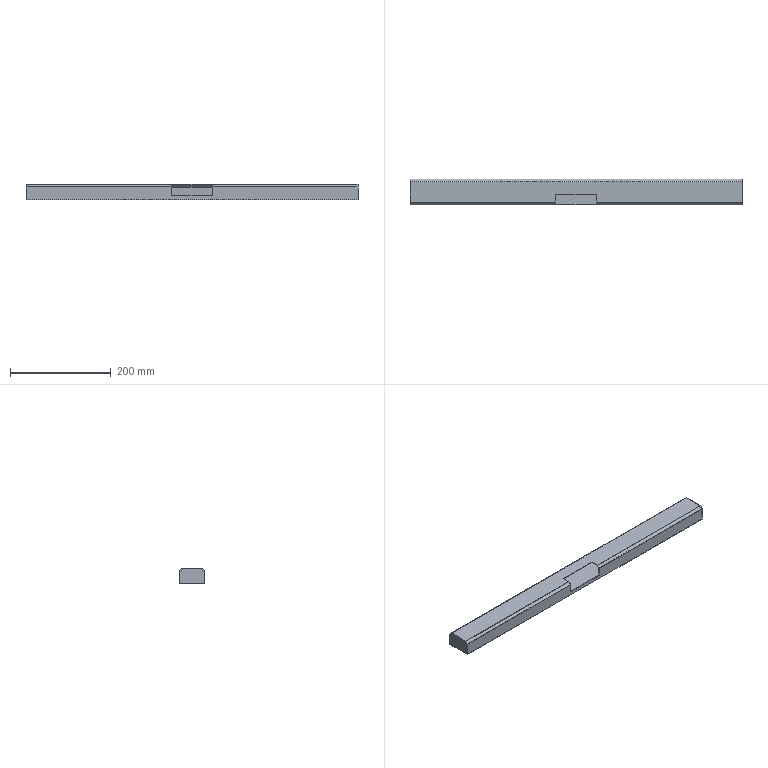Part | STEP file | Guide wheel mechanism revised.sldasm-Part-190 | 1 solid | 22 faces | box 660 x 50 x 30 mm | volume 98910 mm3 | plane 22
STEP:
#1=CARTESIAN_POINT('',(40.,-20.5,108.));
#2=VERTEX_POINT('',#1);
#3=CARTESIAN_POINT('',(40.,-20.5,124.586));
#4=VERTEX_POINT('',#3);
#5=CARTESIAN_POINT('',(40.,-20.5,133.));
#6=DIRECTION('',(0.,0.,1.));
#7=VECTOR('',#6,1000.);
#8=LINE('',#5,#7);
#9=EDGE_CURVE('',#2,#4,#8,.T.);
#10=ORIENTED_EDGE('',*,*,#9,.F.);
#11=CARTESIAN_POINT('',(40.,-21.5,108.));
#12=VERTEX_POINT('',#11);
#13=CARTESIAN_POINT('',(40.,-1.5,108.));
#14=DIRECTION('',(0.,-1.,0.));
#15=VECTOR('',#14,1000.);
#16=LINE('',#13,#15);
#17=EDGE_CURVE('',#2,#12,#16,.T.);
#18=ORIENTED_EDGE('',*,*,#17,.T.);
#19=CARTESIAN_POINT('',(40.,-21.5,125.));
#20=VERTEX_POINT('',#19);
#21=CARTESIAN_POINT('',(40.,-21.5,133.));
#22=DIRECTION('',(0.,0.,1.));
#23=VECTOR('',#22,1000.);
#24=LINE('',#21,#23);
#25=EDGE_CURVE('',#12,#20,#24,.T.);
#26=ORIENTED_EDGE('',*,*,#25,.T.);
#27=CARTESIAN_POINT('',(40.,-16.5,130.));
#28=VERTEX_POINT('',#27);
#29=CARTESIAN_POINT('',(40.,-21.5,125.));
#30=DIRECTION('',(0.,-0.7071,-0.7071));
#31=VECTOR('',#30,1000.);
#32=LINE('',#29,#31);
#33=EDGE_CURVE('',#28,#20,#32,.T.);
#34=ORIENTED_EDGE('',*,*,#33,.F.);
#35=CARTESIAN_POINT('',(40.,-1.5,130.));
#36=VERTEX_POINT('',#35);
#37=CARTESIAN_POINT('',(40.,-16.5,130.));
#38=DIRECTION('',(0.,-1.,0.));
#39=VECTOR('',#38,1000.);
#40=LINE('',#37,#39);
#41=EDGE_CURVE('',#36,#28,#40,.T.);
#42=ORIENTED_EDGE('',*,*,#41,.F.);
#43=CARTESIAN_POINT('',(40.,-1.5,129.));
#44=VERTEX_POINT('',#43);
#45=CARTESIAN_POINT('',(40.,-1.5,133.));
#46=DIRECTION('',(0.,0.,1.));
#47=VECTOR('',#46,1000.);
#48=LINE('',#45,#47);
#49=EDGE_CURVE('',#44,#36,#48,.T.);
#50=ORIENTED_EDGE('',*,*,#49,.F.);
#51=CARTESIAN_POINT('',(40.,-16.086,129.));
#52=VERTEX_POINT('',#51);
#53=CARTESIAN_POINT('',(40.,-16.5,129.));
#54=DIRECTION('',(0.,-1.,0.));
#55=VECTOR('',#54,1000.);
#56=LINE('',#53,#55);
#57=EDGE_CURVE('',#44,#52,#56,.T.);
#58=ORIENTED_EDGE('',*,*,#57,.T.);
#59=CARTESIAN_POINT('',(40.,-20.793,124.293));
#60=DIRECTION('',(0.,-0.7071,-0.7071));
#61=VECTOR('',#60,1000.);
#62=LINE('',#59,#61);
#63=EDGE_CURVE('',#52,#4,#62,.T.);
#64=ORIENTED_EDGE('',*,*,#63,.T.);
#65=EDGE_LOOP('',(#10,#18,#26,#34,#42,#50,#58,#64));
#66=FACE_OUTER_BOUND('',#65,.T.);
#67=CARTESIAN_POINT('',(40.,-1.5,133.));
#68=DIRECTION('',(1.,0.,0.));
#69=DIRECTION('',(0.,0.,-1.));
#70=AXIS2_PLACEMENT_3D('',#67,#68,#69);
#71=PLANE('',#70);
#72=ADVANCED_FACE('',(#66),#71,.F.);
#73=CARTESIAN_POINT('',(-40.,-20.5,108.));
#74=VERTEX_POINT('',#73);
#75=CARTESIAN_POINT('',(-40.,-20.5,108.));
#76=DIRECTION('',(1.,0.,0.));
#77=VECTOR('',#76,1000.);
#78=LINE('',#75,#77);
#79=EDGE_CURVE('',#74,#2,#78,.T.);
#80=ORIENTED_EDGE('',*,*,#79,.F.);
#81=CARTESIAN_POINT('',(-40.,-21.5,108.));
#82=VERTEX_POINT('',#81);
#83=CARTESIAN_POINT('',(-40.,-1.5,108.));
#84=DIRECTION('',(0.,-1.,0.));
#85=VECTOR('',#84,1000.);
#86=LINE('',#83,#85);
#87=EDGE_CURVE('',#74,#82,#86,.T.);
#88=ORIENTED_EDGE('',*,*,#87,.T.);
#89=CARTESIAN_POINT('',(-40.,-21.5,108.));
#90=DIRECTION('',(1.,0.,0.));
#91=VECTOR('',#90,1000.);
#92=LINE('',#89,#91);
#93=EDGE_CURVE('',#82,#12,#92,.T.);
#94=ORIENTED_EDGE('',*,*,#93,.T.);
#95=ORIENTED_EDGE('',*,*,#17,.F.);
#96=EDGE_LOOP('',(#80,#88,#94,#95));
#97=FACE_OUTER_BOUND('',#96,.T.);
#98=CARTESIAN_POINT('',(-40.,-1.5,108.));
#99=DIRECTION('',(0.,0.,-1.));
#100=DIRECTION('',(0.,1.,0.));
#101=AXIS2_PLACEMENT_3D('',#98,#99,#100);
#102=PLANE('',#101);
#103=ADVANCED_FACE('',(#97),#102,.F.);
#104=CARTESIAN_POINT('',(-40.,-21.5,125.));
#105=VERTEX_POINT('',#104);
#106=CARTESIAN_POINT('',(-330.,-21.5,125.));
#107=VERTEX_POINT('',#106);
#108=CARTESIAN_POINT('',(330.,-21.5,125.));
#109=DIRECTION('',(-1.,0.,0.));
#110=VECTOR('',#109,1000.);
#111=LINE('',#108,#110);
#112=EDGE_CURVE('',#105,#107,#111,.T.);
#113=ORIENTED_EDGE('',*,*,#112,.F.);
#114=CARTESIAN_POINT('',(-40.,-16.5,130.));
#115=VERTEX_POINT('',#114);
#116=CARTESIAN_POINT('',(-40.,-21.5,125.));
#117=DIRECTION('',(0.,0.7071,0.7071));
#118=VECTOR('',#117,1000.);
#119=LINE('',#116,#118);
#120=EDGE_CURVE('',#105,#115,#119,.T.);
#121=ORIENTED_EDGE('',*,*,#120,.T.);
#122=CARTESIAN_POINT('',(-330.,-16.5,130.));
#123=VERTEX_POINT('',#122);
#124=CARTESIAN_POINT('',(330.,-16.5,130.));
#125=DIRECTION('',(-1.,0.,0.));
#126=VECTOR('',#125,1000.);
#127=LINE('',#124,#126);
#128=EDGE_CURVE('',#115,#123,#127,.T.);
#129=ORIENTED_EDGE('',*,*,#128,.T.);
#130=CARTESIAN_POINT('',(-330.,-21.5,125.));
#131=DIRECTION('',(0.,-0.7071,-0.7071));
#132=VECTOR('',#131,1000.);
#133=LINE('',#130,#132);
#134=EDGE_CURVE('',#123,#107,#133,.T.);
#135=ORIENTED_EDGE('',*,*,#134,.T.);
#136=EDGE_LOOP('',(#113,#121,#129,#135));
#137=FACE_OUTER_BOUND('',#136,.T.);
#138=CARTESIAN_POINT('',(330.,-21.5,125.));
#139=DIRECTION('',(0.,0.7071,-0.7071));
#140=DIRECTION('',(0.,0.7071,0.7071));
#141=AXIS2_PLACEMENT_3D('',#138,#139,#140);
#142=PLANE('',#141);
#143=ADVANCED_FACE('',(#137),#142,.F.);
#144=CARTESIAN_POINT('',(-330.,28.5,100.));
#145=VERTEX_POINT('',#144);
#146=CARTESIAN_POINT('',(-330.,28.5,125.));
#147=VERTEX_POINT('',#146);
#148=CARTESIAN_POINT('',(-330.,28.5,125.));
#149=DIRECTION('',(0.,0.,1.));
#150=VECTOR('',#149,1000.);
#151=LINE('',#148,#150);
#152=EDGE_CURVE('',#145,#147,#151,.T.);
#153=ORIENTED_EDGE('',*,*,#152,.T.);
#154=CARTESIAN_POINT('',(330.,28.5,125.));
#155=VERTEX_POINT('',#154);
#156=CARTESIAN_POINT('',(330.,28.5,125.));
#157=DIRECTION('',(-1.,0.,0.));
#158=VECTOR('',#157,1000.);
#159=LINE('',#156,#158);
#160=EDGE_CURVE('',#155,#147,#159,.T.);
#161=ORIENTED_EDGE('',*,*,#160,.F.);
#162=CARTESIAN_POINT('',(330.,28.5,100.));
#163=VERTEX_POINT('',#162);
#164=CARTESIAN_POINT('',(330.,28.5,125.));
#165=DIRECTION('',(0.,0.,1.));
#166=VECTOR('',#165,1000.);
#167=LINE('',#164,#166);
#168=EDGE_CURVE('',#163,#155,#167,.T.);
#169=ORIENTED_EDGE('',*,*,#168,.F.);
#170=CARTESIAN_POINT('',(330.,28.5,100.));
#171=DIRECTION('',(-1.,0.,0.));
#172=VECTOR('',#171,1000.);
#173=LINE('',#170,#172);
#174=EDGE_CURVE('',#163,#145,#173,.T.);
#175=ORIENTED_EDGE('',*,*,#174,.T.);
#176=EDGE_LOOP('',(#153,#161,#169,#175));
#177=FACE_OUTER_BOUND('',#176,.T.);
#178=CARTESIAN_POINT('',(330.,28.5,125.));
#179=DIRECTION('',(0.,-1.,0.));
#180=DIRECTION('',(0.,0.,-1.));
#181=AXIS2_PLACEMENT_3D('',#178,#179,#180);
#182=PLANE('',#181);
#183=ADVANCED_FACE('',(#177),#182,.F.);
#184=CARTESIAN_POINT('',(-330.,23.5,130.));
#185=VERTEX_POINT('',#184);
#186=CARTESIAN_POINT('',(-330.,23.5,130.));
#187=DIRECTION('',(0.,-0.7071,0.7071));
#188=VECTOR('',#187,1000.);
#189=LINE('',#186,#188);
#190=EDGE_CURVE('',#147,#185,#189,.T.);
#191=ORIENTED_EDGE('',*,*,#190,.T.);
#192=CARTESIAN_POINT('',(330.,23.5,130.));
#193=VERTEX_POINT('',#192);
#194=CARTESIAN_POINT('',(330.,23.5,130.));
#195=DIRECTION('',(-1.,0.,0.));
#196=VECTOR('',#195,1000.);
#197=LINE('',#194,#196);
#198=EDGE_CURVE('',#193,#185,#197,.T.);
#199=ORIENTED_EDGE('',*,*,#198,.F.);
#200=CARTESIAN_POINT('',(330.,23.5,130.));
#201=DIRECTION('',(0.,-0.7071,0.7071));
#202=VECTOR('',#201,1000.);
#203=LINE('',#200,#202);
#204=EDGE_CURVE('',#155,#193,#203,.T.);
#205=ORIENTED_EDGE('',*,*,#204,.F.);
#206=ORIENTED_EDGE('',*,*,#160,.T.);
#207=EDGE_LOOP('',(#191,#199,#205,#206));
#208=FACE_OUTER_BOUND('',#207,.T.);
#209=CARTESIAN_POINT('',(330.,23.5,130.));
#210=DIRECTION('',(0.,-0.7071,-0.7071));
#211=DIRECTION('',(0.,0.7071,-0.7071));
#212=AXIS2_PLACEMENT_3D('',#209,#210,#211);
#213=PLANE('',#212);
#214=ADVANCED_FACE('',(#208),#213,.F.);
#215=ORIENTED_EDGE('',*,*,#128,.F.);
#216=CARTESIAN_POINT('',(-40.,-1.5,130.));
#217=VERTEX_POINT('',#216);
#218=CARTESIAN_POINT('',(-40.,-16.5,130.));
#219=DIRECTION('',(0.,1.,0.));
#220=VECTOR('',#219,1000.);
#221=LINE('',#218,#220);
#222=EDGE_CURVE('',#115,#217,#221,.T.);
#223=ORIENTED_EDGE('',*,*,#222,.T.);
#224=CARTESIAN_POINT('',(330.,-1.5,130.));
#225=DIRECTION('',(-1.,0.,0.));
#226=VECTOR('',#225,1000.);
#227=LINE('',#224,#226);
#228=EDGE_CURVE('',#36,#217,#227,.T.);
#229=ORIENTED_EDGE('',*,*,#228,.F.);
#230=ORIENTED_EDGE('',*,*,#41,.T.);
#231=CARTESIAN_POINT('',(330.,-16.5,130.));
#232=VERTEX_POINT('',#231);
#233=CARTESIAN_POINT('',(330.,-16.5,130.));
#234=DIRECTION('',(-1.,0.,0.));
#235=VECTOR('',#234,1000.);
#236=LINE('',#233,#235);
#237=EDGE_CURVE('',#232,#28,#236,.T.);
#238=ORIENTED_EDGE('',*,*,#237,.F.);
#239=CARTESIAN_POINT('',(330.,-16.5,130.));
#240=DIRECTION('',(0.,-1.,0.));
#241=VECTOR('',#240,1000.);
#242=LINE('',#239,#241);
#243=EDGE_CURVE('',#193,#232,#242,.T.);
#244=ORIENTED_EDGE('',*,*,#243,.F.);
#245=ORIENTED_EDGE('',*,*,#198,.T.);
#246=CARTESIAN_POINT('',(-330.,-16.5,130.));
#247=DIRECTION('',(0.,-1.,0.));
#248=VECTOR('',#247,1000.);
#249=LINE('',#246,#248);
#250=EDGE_CURVE('',#185,#123,#249,.T.);
#251=ORIENTED_EDGE('',*,*,#250,.T.);
#252=EDGE_LOOP('',(#215,#223,#229,#230,#238,#244,#245,#251));
#253=FACE_OUTER_BOUND('',#252,.T.);
#254=CARTESIAN_POINT('',(330.,-16.5,130.));
#255=DIRECTION('',(0.,0.,-1.));
#256=DIRECTION('',(0.,1.,0.));
#257=AXIS2_PLACEMENT_3D('',#254,#255,#256);
#258=PLANE('',#257);
#259=ADVANCED_FACE('',(#253),#258,.F.);
#260=ORIENTED_EDGE('',*,*,#237,.T.);
#261=ORIENTED_EDGE('',*,*,#33,.T.);
#262=CARTESIAN_POINT('',(330.,-21.5,125.));
#263=VERTEX_POINT('',#262);
#264=CARTESIAN_POINT('',(330.,-21.5,125.));
#265=DIRECTION('',(-1.,0.,0.));
#266=VECTOR('',#265,1000.);
#267=LINE('',#264,#266);
#268=EDGE_CURVE('',#263,#20,#267,.T.);
#269=ORIENTED_EDGE('',*,*,#268,.F.);
#270=CARTESIAN_POINT('',(330.,-21.5,125.));
#271=DIRECTION('',(0.,-0.7071,-0.7071));
#272=VECTOR('',#271,1000.);
#273=LINE('',#270,#272);
#274=EDGE_CURVE('',#232,#263,#273,.T.);
#275=ORIENTED_EDGE('',*,*,#274,.F.);
#276=EDGE_LOOP('',(#260,#261,#269,#275));
#277=FACE_OUTER_BOUND('',#276,.T.);
#278=CARTESIAN_POINT('',(330.,-21.5,125.));
#279=DIRECTION('',(0.,0.7071,-0.7071));
#280=DIRECTION('',(0.,0.7071,0.7071));
#281=AXIS2_PLACEMENT_3D('',#278,#279,#280);
#282=PLANE('',#281);
#283=ADVANCED_FACE('',(#277),#282,.F.);
#284=ORIENTED_EDGE('',*,*,#93,.F.);
#285=CARTESIAN_POINT('',(-40.,-21.5,100.));
#286=DIRECTION('',(0.,0.,1.));
#287=VECTOR('',#286,1000.);
#288=LINE('',#285,#287);
#289=EDGE_CURVE('',#82,#105,#288,.T.);
#290=ORIENTED_EDGE('',*,*,#289,.T.);
#291=ORIENTED_EDGE('',*,*,#112,.T.);
#292=CARTESIAN_POINT('',(-330.,-21.5,100.));
#293=VERTEX_POINT('',#292);
#294=CARTESIAN_POINT('',(-330.,-21.5,100.));
#295=DIRECTION('',(0.,0.,-1.));
#296=VECTOR('',#295,1000.);
#297=LINE('',#294,#296);
#298=EDGE_CURVE('',#107,#293,#297,.T.);
#299=ORIENTED_EDGE('',*,*,#298,.T.);
#300=CARTESIAN_POINT('',(330.,-21.5,100.));
#301=VERTEX_POINT('',#300);
#302=CARTESIAN_POINT('',(330.,-21.5,100.));
#303=DIRECTION('',(-1.,0.,0.));
#304=VECTOR('',#303,1000.);
#305=LINE('',#302,#304);
#306=EDGE_CURVE('',#301,#293,#305,.T.);
#307=ORIENTED_EDGE('',*,*,#306,.F.);
#308=CARTESIAN_POINT('',(330.,-21.5,100.));
#309=DIRECTION('',(0.,0.,-1.));
#310=VECTOR('',#309,1000.);
#311=LINE('',#308,#310);
#312=EDGE_CURVE('',#263,#301,#311,.T.);
#313=ORIENTED_EDGE('',*,*,#312,.F.);
#314=ORIENTED_EDGE('',*,*,#268,.T.);
#315=ORIENTED_EDGE('',*,*,#25,.F.);
#316=EDGE_LOOP('',(#284,#290,#291,#299,#307,#313,#314,#315));
#317=FACE_OUTER_BOUND('',#316,.T.);
#318=CARTESIAN_POINT('',(330.,-21.5,100.));
#319=DIRECTION('',(0.,1.,0.));
#320=DIRECTION('',(0.,0.,1.));
#321=AXIS2_PLACEMENT_3D('',#318,#319,#320);
#322=PLANE('',#321);
#323=ADVANCED_FACE('',(#317),#322,.F.);
#324=CARTESIAN_POINT('',(-330.,28.5,100.));
#325=DIRECTION('',(0.,1.,0.));
#326=VECTOR('',#325,1000.);
#327=LINE('',#324,#326);
#328=EDGE_CURVE('',#293,#145,#327,.T.);
#329=ORIENTED_EDGE('',*,*,#328,.T.);
#330=ORIENTED_EDGE('',*,*,#174,.F.);
#331=CARTESIAN_POINT('',(330.,28.5,100.));
#332=DIRECTION('',(0.,1.,0.));
#333=VECTOR('',#332,1000.);
#334=LINE('',#331,#333);
#335=EDGE_CURVE('',#301,#163,#334,.T.);
#336=ORIENTED_EDGE('',*,*,#335,.F.);
#337=ORIENTED_EDGE('',*,*,#306,.T.);
#338=EDGE_LOOP('',(#329,#330,#336,#337));
#339=FACE_OUTER_BOUND('',#338,.T.);
#340=CARTESIAN_POINT('',(330.,28.5,100.));
#341=DIRECTION('',(0.,0.,1.));
#342=DIRECTION('',(0.,-1.,0.));
#343=AXIS2_PLACEMENT_3D('',#340,#341,#342);
#344=PLANE('',#343);
#345=ADVANCED_FACE('',(#339),#344,.F.);
#346=ORIENTED_EDGE('',*,*,#168,.T.);
#347=ORIENTED_EDGE('',*,*,#204,.T.);
#348=ORIENTED_EDGE('',*,*,#243,.T.);
#349=ORIENTED_EDGE('',*,*,#274,.T.);
#350=ORIENTED_EDGE('',*,*,#312,.T.);
#351=ORIENTED_EDGE('',*,*,#335,.T.);
#352=EDGE_LOOP('',(#346,#347,#348,#349,#350,#351));
#353=FACE_OUTER_BOUND('',#352,.T.);
#354=CARTESIAN_POINT('',(330.,28.5,100.));
#355=DIRECTION('',(-1.,0.,0.));
#356=DIRECTION('',(0.,0.,1.));
#357=AXIS2_PLACEMENT_3D('',#354,#355,#356);
#358=PLANE('',#357);
#359=ADVANCED_FACE('',(#353),#358,.F.);
#360=ORIENTED_EDGE('',*,*,#152,.F.);
#361=ORIENTED_EDGE('',*,*,#328,.F.);
#362=ORIENTED_EDGE('',*,*,#298,.F.);
#363=ORIENTED_EDGE('',*,*,#134,.F.);
#364=ORIENTED_EDGE('',*,*,#250,.F.);
#365=ORIENTED_EDGE('',*,*,#190,.F.);
#366=EDGE_LOOP('',(#360,#361,#362,#363,#364,#365));
#367=FACE_OUTER_BOUND('',#366,.T.);
#368=CARTESIAN_POINT('',(-330.,28.5,100.));
#369=DIRECTION('',(-1.,0.,0.));
#370=DIRECTION('',(0.,0.,1.));
#371=AXIS2_PLACEMENT_3D('',#368,#369,#370);
#372=PLANE('',#371);
#373=ADVANCED_FACE('',(#367),#372,.T.);
#374=CARTESIAN_POINT('',(-40.,-1.5,129.));
#375=VERTEX_POINT('',#374);
#376=CARTESIAN_POINT('',(330.,-1.5,129.));
#377=DIRECTION('',(-1.,0.,0.));
#378=VECTOR('',#377,1000.);
#379=LINE('',#376,#378);
#380=EDGE_CURVE('',#44,#375,#379,.T.);
#381=ORIENTED_EDGE('',*,*,#380,.F.);
#382=ORIENTED_EDGE('',*,*,#49,.T.);
#383=ORIENTED_EDGE('',*,*,#228,.T.);
#384=CARTESIAN_POINT('',(-40.,-1.5,133.));
#385=DIRECTION('',(0.,0.,-1.));
#386=VECTOR('',#385,1000.);
#387=LINE('',#384,#386);
#388=EDGE_CURVE('',#217,#375,#387,.T.);
#389=ORIENTED_EDGE('',*,*,#388,.T.);
#390=EDGE_LOOP('',(#381,#382,#383,#389));
#391=FACE_OUTER_BOUND('',#390,.T.);
#392=CARTESIAN_POINT('',(-40.,-1.5,108.));
#393=DIRECTION('',(0.,-1.,0.));
#394=DIRECTION('',(0.,0.,-1.));
#395=AXIS2_PLACEMENT_3D('',#392,#393,#394);
#396=PLANE('',#395);
#397=ADVANCED_FACE('',(#391),#396,.T.);
#398=ORIENTED_EDGE('',*,*,#87,.F.);
#399=CARTESIAN_POINT('',(-40.,-20.5,124.586));
#400=VERTEX_POINT('',#399);
#401=CARTESIAN_POINT('',(-40.,-20.5,100.));
#402=DIRECTION('',(0.,0.,1.));
#403=VECTOR('',#402,1000.);
#404=LINE('',#401,#403);
#405=EDGE_CURVE('',#74,#400,#404,.T.);
#406=ORIENTED_EDGE('',*,*,#405,.T.);
#407=CARTESIAN_POINT('',(-40.,-16.086,129.));
#408=VERTEX_POINT('',#407);
#409=CARTESIAN_POINT('',(-40.,-20.793,124.293));
#410=DIRECTION('',(0.,0.7071,0.7071));
#411=VECTOR('',#410,1000.);
#412=LINE('',#409,#411);
#413=EDGE_CURVE('',#400,#408,#412,.T.);
#414=ORIENTED_EDGE('',*,*,#413,.T.);
#415=CARTESIAN_POINT('',(-40.,-16.5,129.));
#416=DIRECTION('',(0.,1.,0.));
#417=VECTOR('',#416,1000.);
#418=LINE('',#415,#417);
#419=EDGE_CURVE('',#408,#375,#418,.T.);
#420=ORIENTED_EDGE('',*,*,#419,.T.);
#421=ORIENTED_EDGE('',*,*,#388,.F.);
#422=ORIENTED_EDGE('',*,*,#222,.F.);
#423=ORIENTED_EDGE('',*,*,#120,.F.);
#424=ORIENTED_EDGE('',*,*,#289,.F.);
#425=EDGE_LOOP('',(#398,#406,#414,#420,#421,#422,#423,#424));
#426=FACE_OUTER_BOUND('',#425,.T.);
#427=CARTESIAN_POINT('',(-40.,-1.5,133.));
#428=DIRECTION('',(-1.,0.,0.));
#429=DIRECTION('',(0.,0.,1.));
#430=AXIS2_PLACEMENT_3D('',#427,#428,#429);
#431=PLANE('',#430);
#432=ADVANCED_FACE('',(#426),#431,.F.);
#433=CARTESIAN_POINT('',(-329.,-20.5,124.586));
#434=VERTEX_POINT('',#433);
#435=CARTESIAN_POINT('',(330.,-20.5,124.586));
#436=DIRECTION('',(-1.,0.,0.));
#437=VECTOR('',#436,1000.);
#438=LINE('',#435,#437);
#439=EDGE_CURVE('',#400,#434,#438,.T.);
#440=ORIENTED_EDGE('',*,*,#439,.T.);
#441=CARTESIAN_POINT('',(-329.,-16.086,129.));
#442=VERTEX_POINT('',#441);
#443=CARTESIAN_POINT('',(-329.,-8.293,136.793));
#444=DIRECTION('',(0.,-0.7071,-0.7071));
#445=VECTOR('',#444,1000.);
#446=LINE('',#443,#445);
#447=EDGE_CURVE('',#442,#434,#446,.T.);
#448=ORIENTED_EDGE('',*,*,#447,.F.);
#449=CARTESIAN_POINT('',(330.,-16.086,129.));
#450=DIRECTION('',(-1.,0.,0.));
#451=VECTOR('',#450,1000.);
#452=LINE('',#449,#451);
#453=EDGE_CURVE('',#408,#442,#452,.T.);
#454=ORIENTED_EDGE('',*,*,#453,.F.);
#455=ORIENTED_EDGE('',*,*,#413,.F.);
#456=EDGE_LOOP('',(#440,#448,#454,#455));
#457=FACE_OUTER_BOUND('',#456,.T.);
#458=CARTESIAN_POINT('',(330.,-20.793,124.293));
#459=DIRECTION('',(0.,0.7071,-0.7071));
#460=DIRECTION('',(0.,0.7071,0.7071));
#461=AXIS2_PLACEMENT_3D('',#458,#459,#460);
#462=PLANE('',#461);
#463=ADVANCED_FACE('',(#457),#462,.T.);
#464=CARTESIAN_POINT('',(-329.,27.5,101.));
#465=VERTEX_POINT('',#464);
#466=CARTESIAN_POINT('',(-329.,27.5,124.586));
#467=VERTEX_POINT('',#466);
#468=CARTESIAN_POINT('',(-329.,27.5,100.));
#469=DIRECTION('',(0.,0.,1.));
#470=VECTOR('',#469,1000.);
#471=LINE('',#468,#470);
#472=EDGE_CURVE('',#465,#467,#471,.T.);
#473=ORIENTED_EDGE('',*,*,#472,.F.);
#474=CARTESIAN_POINT('',(329.,27.5,101.));
#475=VERTEX_POINT('',#474);
#476=CARTESIAN_POINT('',(330.,27.5,101.));
#477=DIRECTION('',(-1.,0.,0.));
#478=VECTOR('',#477,1000.);
#479=LINE('',#476,#478);
#480=EDGE_CURVE('',#475,#465,#479,.T.);
#481=ORIENTED_EDGE('',*,*,#480,.F.);
#482=CARTESIAN_POINT('',(329.,27.5,124.586));
#483=VERTEX_POINT('',#482);
#484=CARTESIAN_POINT('',(329.,27.5,100.));
#485=DIRECTION('',(0.,0.,1.));
#486=VECTOR('',#485,1000.);
#487=LINE('',#484,#486);
#488=EDGE_CURVE('',#475,#483,#487,.T.);
#489=ORIENTED_EDGE('',*,*,#488,.T.);
#490=CARTESIAN_POINT('',(330.,27.5,124.586));
#491=DIRECTION('',(-1.,0.,0.));
#492=VECTOR('',#491,1000.);
#493=LINE('',#490,#492);
#494=EDGE_CURVE('',#483,#467,#493,.T.);
#495=ORIENTED_EDGE('',*,*,#494,.T.);
#496=EDGE_LOOP('',(#473,#481,#489,#495));
#497=FACE_OUTER_BOUND('',#496,.T.);
#498=CARTESIAN_POINT('',(330.,27.5,125.));
#499=DIRECTION('',(0.,-1.,0.));
#500=DIRECTION('',(0.,0.,-1.));
#501=AXIS2_PLACEMENT_3D('',#498,#499,#500);
#502=PLANE('',#501);
#503=ADVANCED_FACE('',(#497),#502,.T.);
#504=CARTESIAN_POINT('',(-329.,23.086,129.));
#505=VERTEX_POINT('',#504);
#506=CARTESIAN_POINT('',(-329.,40.293,111.793));
#507=DIRECTION('',(0.,-0.7071,0.7071));
#508=VECTOR('',#507,1000.);
#509=LINE('',#506,#508);
#510=EDGE_CURVE('',#467,#505,#509,.T.);
#511=ORIENTED_EDGE('',*,*,#510,.F.);
#512=ORIENTED_EDGE('',*,*,#494,.F.);
#513=CARTESIAN_POINT('',(329.,23.086,129.));
#514=VERTEX_POINT('',#513);
#515=CARTESIAN_POINT('',(329.,40.293,111.793));
#516=DIRECTION('',(0.,-0.7071,0.7071));
#517=VECTOR('',#516,1000.);
#518=LINE('',#515,#517);
#519=EDGE_CURVE('',#483,#514,#518,.T.);
#520=ORIENTED_EDGE('',*,*,#519,.T.);
#521=CARTESIAN_POINT('',(330.,23.086,129.));
#522=DIRECTION('',(-1.,0.,0.));
#523=VECTOR('',#522,1000.);
#524=LINE('',#521,#523);
#525=EDGE_CURVE('',#514,#505,#524,.T.);
#526=ORIENTED_EDGE('',*,*,#525,.T.);
#527=EDGE_LOOP('',(#511,#512,#520,#526));
#528=FACE_OUTER_BOUND('',#527,.T.);
#529=CARTESIAN_POINT('',(330.,22.793,129.293));
#530=DIRECTION('',(0.,-0.7071,-0.7071));
#531=DIRECTION('',(0.,0.7071,-0.7071));
#532=AXIS2_PLACEMENT_3D('',#529,#530,#531);
#533=PLANE('',#532);
#534=ADVANCED_FACE('',(#528),#533,.T.);
#535=ORIENTED_EDGE('',*,*,#453,.T.);
#536=CARTESIAN_POINT('',(-329.,28.5,129.));
#537=DIRECTION('',(0.,-1.,0.));
#538=VECTOR('',#537,1000.);
#539=LINE('',#536,#538);
#540=EDGE_CURVE('',#505,#442,#539,.T.);
#541=ORIENTED_EDGE('',*,*,#540,.F.);
#542=ORIENTED_EDGE('',*,*,#525,.F.);
#543=CARTESIAN_POINT('',(329.,-16.086,129.));
#544=VERTEX_POINT('',#543);
#545=CARTESIAN_POINT('',(329.,28.5,129.));
#546=DIRECTION('',(0.,-1.,0.));
#547=VECTOR('',#546,1000.);
#548=LINE('',#545,#547);
#549=EDGE_CURVE('',#514,#544,#548,.T.);
#550=ORIENTED_EDGE('',*,*,#549,.T.);
#551=CARTESIAN_POINT('',(330.,-16.086,129.));
#552=DIRECTION('',(-1.,0.,0.));
#553=VECTOR('',#552,1000.);
#554=LINE('',#551,#553);
#555=EDGE_CURVE('',#544,#52,#554,.T.);
#556=ORIENTED_EDGE('',*,*,#555,.T.);
#557=ORIENTED_EDGE('',*,*,#57,.F.);
#558=ORIENTED_EDGE('',*,*,#380,.T.);
#559=ORIENTED_EDGE('',*,*,#419,.F.);
#560=EDGE_LOOP('',(#535,#541,#542,#550,#556,#557,#558,#559));
#561=FACE_OUTER_BOUND('',#560,.T.);
#562=CARTESIAN_POINT('',(330.,-16.5,129.));
#563=DIRECTION('',(0.,0.,-1.));
#564=DIRECTION('',(0.,1.,0.));
#565=AXIS2_PLACEMENT_3D('',#562,#563,#564);
#566=PLANE('',#565);
#567=ADVANCED_FACE('',(#561),#566,.T.);
#568=ORIENTED_EDGE('',*,*,#555,.F.);
#569=CARTESIAN_POINT('',(329.,-20.5,124.586));
#570=VERTEX_POINT('',#569);
#571=CARTESIAN_POINT('',(329.,-8.293,136.793));
#572=DIRECTION('',(0.,-0.7071,-0.7071));
#573=VECTOR('',#572,1000.);
#574=LINE('',#571,#573);
#575=EDGE_CURVE('',#544,#570,#574,.T.);
#576=ORIENTED_EDGE('',*,*,#575,.T.);
#577=CARTESIAN_POINT('',(330.,-20.5,124.586));
#578=DIRECTION('',(-1.,0.,0.));
#579=VECTOR('',#578,1000.);
#580=LINE('',#577,#579);
#581=EDGE_CURVE('',#570,#4,#580,.T.);
#582=ORIENTED_EDGE('',*,*,#581,.T.);
#583=ORIENTED_EDGE('',*,*,#63,.F.);
#584=EDGE_LOOP('',(#568,#576,#582,#583));
#585=FACE_OUTER_BOUND('',#584,.T.);
#586=CARTESIAN_POINT('',(330.,-20.793,124.293));
#587=DIRECTION('',(0.,0.7071,-0.7071));
#588=DIRECTION('',(0.,0.7071,0.7071));
#589=AXIS2_PLACEMENT_3D('',#586,#587,#588);
#590=PLANE('',#589);
#591=ADVANCED_FACE('',(#585),#590,.T.);
#592=ORIENTED_EDGE('',*,*,#79,.T.);
#593=ORIENTED_EDGE('',*,*,#9,.T.);
#594=ORIENTED_EDGE('',*,*,#581,.F.);
#595=CARTESIAN_POINT('',(329.,-20.5,101.));
#596=VERTEX_POINT('',#595);
#597=CARTESIAN_POINT('',(329.,-20.5,100.));
#598=DIRECTION('',(0.,0.,-1.));
#599=VECTOR('',#598,1000.);
#600=LINE('',#597,#599);
#601=EDGE_CURVE('',#570,#596,#600,.T.);
#602=ORIENTED_EDGE('',*,*,#601,.T.);
#603=CARTESIAN_POINT('',(-329.,-20.5,101.));
#604=VERTEX_POINT('',#603);
#605=CARTESIAN_POINT('',(330.,-20.5,101.));
#606=DIRECTION('',(-1.,0.,0.));
#607=VECTOR('',#606,1000.);
#608=LINE('',#605,#607);
#609=EDGE_CURVE('',#596,#604,#608,.T.);
#610=ORIENTED_EDGE('',*,*,#609,.T.);
#611=CARTESIAN_POINT('',(-329.,-20.5,100.));
#612=DIRECTION('',(0.,0.,-1.));
#613=VECTOR('',#612,1000.);
#614=LINE('',#611,#613);
#615=EDGE_CURVE('',#434,#604,#614,.T.);
#616=ORIENTED_EDGE('',*,*,#615,.F.);
#617=ORIENTED_EDGE('',*,*,#439,.F.);
#618=ORIENTED_EDGE('',*,*,#405,.F.);
#619=EDGE_LOOP('',(#592,#593,#594,#602,#610,#616,#617,#618));
#620=FACE_OUTER_BOUND('',#619,.T.);
#621=CARTESIAN_POINT('',(330.,-20.5,100.));
#622=DIRECTION('',(0.,1.,0.));
#623=DIRECTION('',(0.,0.,1.));
#624=AXIS2_PLACEMENT_3D('',#621,#622,#623);
#625=PLANE('',#624);
#626=ADVANCED_FACE('',(#620),#625,.T.);
#627=CARTESIAN_POINT('',(-329.,28.5,101.));
#628=DIRECTION('',(0.,1.,0.));
#629=VECTOR('',#628,1000.);
#630=LINE('',#627,#629);
#631=EDGE_CURVE('',#604,#465,#630,.T.);
#632=ORIENTED_EDGE('',*,*,#631,.F.);
#633=ORIENTED_EDGE('',*,*,#609,.F.);
#634=CARTESIAN_POINT('',(329.,28.5,101.));
#635=DIRECTION('',(0.,1.,0.));
#636=VECTOR('',#635,1000.);
#637=LINE('',#634,#636);
#638=EDGE_CURVE('',#596,#475,#637,.T.);
#639=ORIENTED_EDGE('',*,*,#638,.T.);
#640=ORIENTED_EDGE('',*,*,#480,.T.);
#641=EDGE_LOOP('',(#632,#633,#639,#640));
#642=FACE_OUTER_BOUND('',#641,.T.);
#643=CARTESIAN_POINT('',(330.,28.5,101.));
#644=DIRECTION('',(0.,0.,1.));
#645=DIRECTION('',(0.,-1.,0.));
#646=AXIS2_PLACEMENT_3D('',#643,#644,#645);
#647=PLANE('',#646);
#648=ADVANCED_FACE('',(#642),#647,.T.);
#649=ORIENTED_EDGE('',*,*,#488,.F.);
#650=ORIENTED_EDGE('',*,*,#638,.F.);
#651=ORIENTED_EDGE('',*,*,#601,.F.);
#652=ORIENTED_EDGE('',*,*,#575,.F.);
#653=ORIENTED_EDGE('',*,*,#549,.F.);
#654=ORIENTED_EDGE('',*,*,#519,.F.);
#655=EDGE_LOOP('',(#649,#650,#651,#652,#653,#654));
#656=FACE_OUTER_BOUND('',#655,.T.);
#657=CARTESIAN_POINT('',(329.,28.5,100.));
#658=DIRECTION('',(-1.,0.,0.));
#659=DIRECTION('',(0.,0.,1.));
#660=AXIS2_PLACEMENT_3D('',#657,#658,#659);
#661=PLANE('',#660);
#662=ADVANCED_FACE('',(#656),#661,.T.);
#663=ORIENTED_EDGE('',*,*,#472,.T.);
#664=ORIENTED_EDGE('',*,*,#510,.T.);
#665=ORIENTED_EDGE('',*,*,#540,.T.);
#666=ORIENTED_EDGE('',*,*,#447,.T.);
#667=ORIENTED_EDGE('',*,*,#615,.T.);
#668=ORIENTED_EDGE('',*,*,#631,.T.);
#669=EDGE_LOOP('',(#663,#664,#665,#666,#667,#668));
#670=FACE_OUTER_BOUND('',#669,.T.);
#671=CARTESIAN_POINT('',(-329.,28.5,100.));
#672=DIRECTION('',(-1.,0.,0.));
#673=DIRECTION('',(0.,0.,1.));
#674=AXIS2_PLACEMENT_3D('',#671,#672,#673);
#675=PLANE('',#674);
#676=ADVANCED_FACE('',(#670),#675,.F.);
#677=CLOSED_SHELL('',(#72,#103,#143,#183,#214,#259,#283,#323,#345,#359,#373,#397,#432,#463,#503,#534,#567,#591,#626,#648,#662,#676));
#678=MANIFOLD_SOLID_BREP('',#677);
#679=CARTESIAN_POINT('',(0.,0.,0.));
#680=DIRECTION('',(0.,0.,1.));
#681=DIRECTION('',(1.,0.,0.));
#682=AXIS2_PLACEMENT_3D('',#679,#680,#681);
#683=(LENGTH_UNIT()NAMED_UNIT(*)SI_UNIT(.MILLI.,.METRE.));
#684=UNCERTAINTY_MEASURE_WITH_UNIT(LENGTH_MEASURE(0.00001),#683,'','');
#685=(NAMED_UNIT(*)PLANE_ANGLE_UNIT()SI_UNIT($,.RADIAN.));
#686=(NAMED_UNIT(*)SI_UNIT($,.STERADIAN.)SOLID_ANGLE_UNIT());
#687=(GEOMETRIC_REPRESENTATION_CONTEXT(3)GLOBAL_UNCERTAINTY_ASSIGNED_CONTEXT((#684))GLOBAL_UNIT_ASSIGNED_CONTEXT((#683,#685,#686))REPRESENTATION_CONTEXT('',''));
#688=ADVANCED_BREP_SHAPE_REPRESENTATION('',(#678,#682),#687);